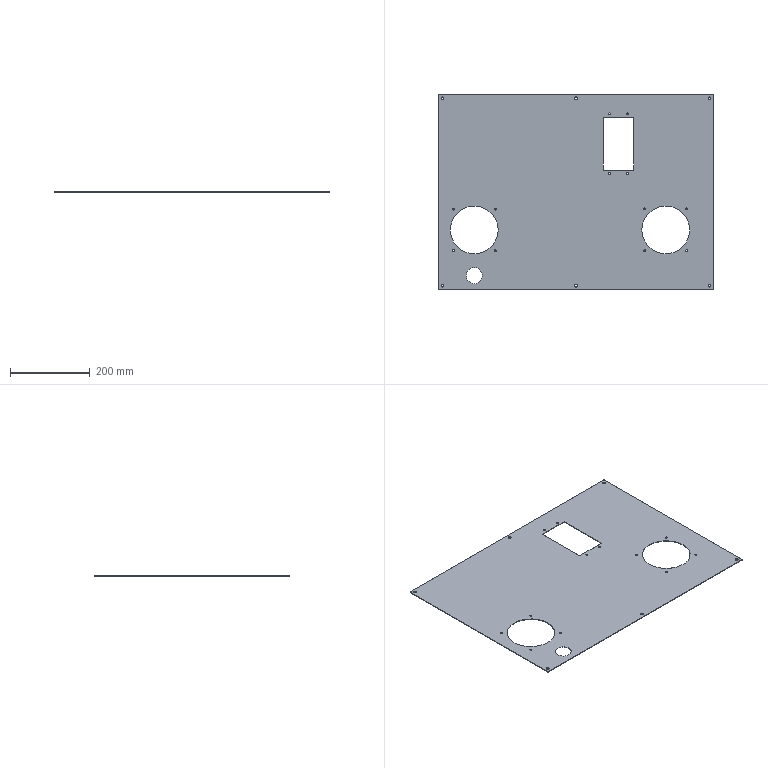Part | NX | 1 solid | 60 faces | box 690 x 490 x 1.5 mm | volume 455384 mm3 | cylinder 46 | plane 10 | cone 4 | commonest cylinder face diameters 5 x24 7 x12 4 x4 120 x4 40 x2